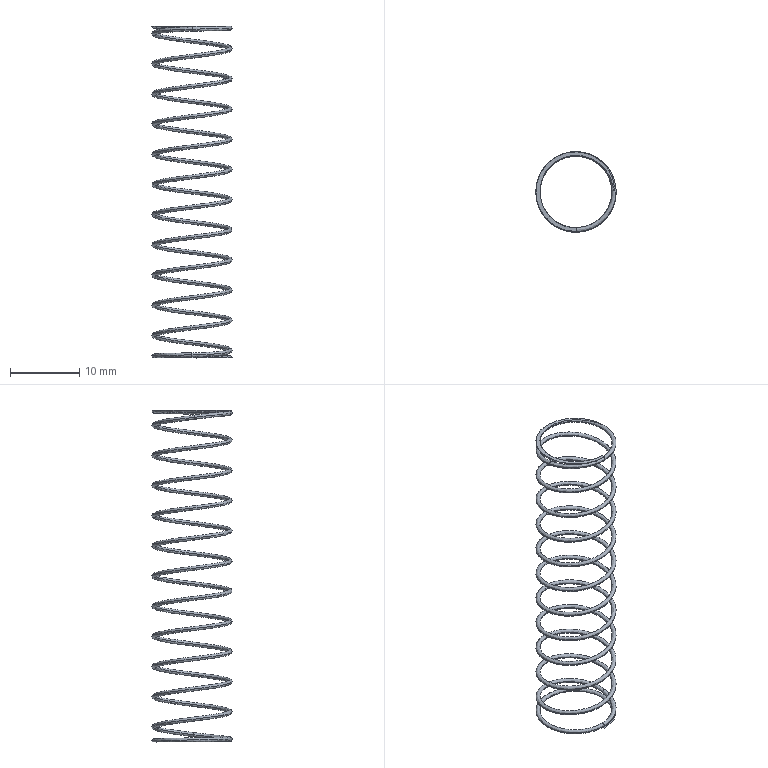Part | SolidWorks | features BaseBody 1 | 1 solid | 14 faces | volume 116.54 mm3 | spline 10 | plane 4